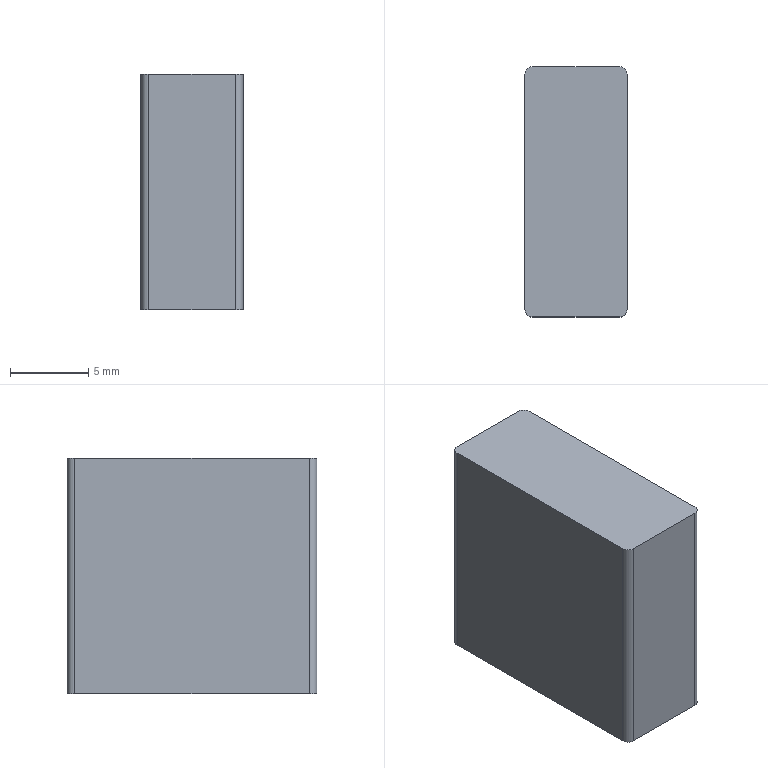Part | NX | features BREP 1 | 1 solid | 10 faces | box 6.52 x 15.946 x 15 mm | volume 1556 mm3 | plane 6 | cylinder 4 | commonest cylinder face diameters 1 x4
STEP:
#1=CARTESIAN_POINT('',(-2.76,7.973,-25.6));
#2=VERTEX_POINT('',#1);
#3=CARTESIAN_POINT('',(-3.26,7.473,-25.6));
#4=VERTEX_POINT('',#3);
#5=CARTESIAN_POINT('',(-2.76,7.473,-25.6));
#6=DIRECTION('',(0.,0.,1.));
#7=DIRECTION('',(1.,0.,0.));
#8=AXIS2_PLACEMENT_3D('',#5,#6,#7);
#9=CIRCLE('',#8,0.5);
#10=EDGE_CURVE('',#2,#4,#9,.T.);
#11=ORIENTED_EDGE('',*,*,#10,.F.);
#12=CARTESIAN_POINT('',(-2.76,7.973,-40.6));
#13=VERTEX_POINT('',#12);
#14=CARTESIAN_POINT('',(-2.76,7.973,-40.6));
#15=DIRECTION('',(0.,0.,1.));
#16=VECTOR('',#15,1000.);
#17=LINE('',#14,#16);
#18=EDGE_CURVE('',#13,#2,#17,.T.);
#19=ORIENTED_EDGE('',*,*,#18,.F.);
#20=CARTESIAN_POINT('',(-3.26,7.473,-40.6));
#21=VERTEX_POINT('',#20);
#22=CARTESIAN_POINT('',(-2.76,7.473,-40.6));
#23=DIRECTION('',(0.,0.,1.));
#24=DIRECTION('',(1.,0.,0.));
#25=AXIS2_PLACEMENT_3D('',#22,#23,#24);
#26=CIRCLE('',#25,0.5);
#27=EDGE_CURVE('',#13,#21,#26,.T.);
#28=ORIENTED_EDGE('',*,*,#27,.T.);
#29=CARTESIAN_POINT('',(-3.26,7.473,-40.6));
#30=DIRECTION('',(0.,0.,1.));
#31=VECTOR('',#30,1000.);
#32=LINE('',#29,#31);
#33=EDGE_CURVE('',#21,#4,#32,.T.);
#34=ORIENTED_EDGE('',*,*,#33,.T.);
#35=EDGE_LOOP('',(#11,#19,#28,#34));
#36=FACE_BOUND('',#35,.T.);
#37=CARTESIAN_POINT('',(-2.76,7.473,-40.6));
#38=DIRECTION('',(0.,0.,1.));
#39=DIRECTION('',(-1.,0.,0.));
#40=AXIS2_PLACEMENT_3D('',#37,#38,#39);
#41=CYLINDRICAL_SURFACE('',#40,0.5);
#42=ADVANCED_FACE('',(#36),#41,.T.);
#43=CARTESIAN_POINT('',(-3.26,-7.473,-25.6));
#44=VERTEX_POINT('',#43);
#45=CARTESIAN_POINT('',(-3.26,-7.473,-25.6));
#46=DIRECTION('',(0.,1.,0.));
#47=VECTOR('',#46,1000.);
#48=LINE('',#45,#47);
#49=EDGE_CURVE('',#44,#4,#48,.T.);
#50=ORIENTED_EDGE('',*,*,#49,.T.);
#51=ORIENTED_EDGE('',*,*,#33,.F.);
#52=CARTESIAN_POINT('',(-3.26,-7.473,-40.6));
#53=VERTEX_POINT('',#52);
#54=CARTESIAN_POINT('',(-3.26,-7.473,-40.6));
#55=DIRECTION('',(0.,1.,0.));
#56=VECTOR('',#55,1000.);
#57=LINE('',#54,#56);
#58=EDGE_CURVE('',#53,#21,#57,.T.);
#59=ORIENTED_EDGE('',*,*,#58,.F.);
#60=CARTESIAN_POINT('',(-3.26,-7.473,-40.6));
#61=DIRECTION('',(0.,0.,1.));
#62=VECTOR('',#61,1000.);
#63=LINE('',#60,#62);
#64=EDGE_CURVE('',#53,#44,#63,.T.);
#65=ORIENTED_EDGE('',*,*,#64,.T.);
#66=EDGE_LOOP('',(#50,#51,#59,#65));
#67=FACE_BOUND('',#66,.T.);
#68=CARTESIAN_POINT('',(-3.26,-7.473,-40.6));
#69=DIRECTION('',(1.,0.,0.));
#70=DIRECTION('',(0.,-1.,0.));
#71=AXIS2_PLACEMENT_3D('',#68,#69,#70);
#72=PLANE('',#71);
#73=ADVANCED_FACE('',(#67),#72,.F.);
#74=CARTESIAN_POINT('',(-2.76,-7.973,-25.6));
#75=VERTEX_POINT('',#74);
#76=CARTESIAN_POINT('',(-2.76,-7.473,-25.6));
#77=DIRECTION('',(0.,0.,1.));
#78=DIRECTION('',(1.,0.,0.));
#79=AXIS2_PLACEMENT_3D('',#76,#77,#78);
#80=CIRCLE('',#79,0.5);
#81=EDGE_CURVE('',#44,#75,#80,.T.);
#82=ORIENTED_EDGE('',*,*,#81,.F.);
#83=ORIENTED_EDGE('',*,*,#64,.F.);
#84=CARTESIAN_POINT('',(-2.76,-7.973,-40.6));
#85=VERTEX_POINT('',#84);
#86=CARTESIAN_POINT('',(-2.76,-7.473,-40.6));
#87=DIRECTION('',(0.,0.,1.));
#88=DIRECTION('',(1.,0.,0.));
#89=AXIS2_PLACEMENT_3D('',#86,#87,#88);
#90=CIRCLE('',#89,0.5);
#91=EDGE_CURVE('',#53,#85,#90,.T.);
#92=ORIENTED_EDGE('',*,*,#91,.T.);
#93=CARTESIAN_POINT('',(-2.76,-7.973,-40.6));
#94=DIRECTION('',(0.,0.,1.));
#95=VECTOR('',#94,1000.);
#96=LINE('',#93,#95);
#97=EDGE_CURVE('',#85,#75,#96,.T.);
#98=ORIENTED_EDGE('',*,*,#97,.T.);
#99=EDGE_LOOP('',(#82,#83,#92,#98));
#100=FACE_BOUND('',#99,.T.);
#101=CARTESIAN_POINT('',(-2.76,-7.473,-40.6));
#102=DIRECTION('',(0.,0.,1.));
#103=DIRECTION('',(-1.,0.,0.));
#104=AXIS2_PLACEMENT_3D('',#101,#102,#103);
#105=CYLINDRICAL_SURFACE('',#104,0.5);
#106=ADVANCED_FACE('',(#100),#105,.T.);
#107=CARTESIAN_POINT('',(2.76,-7.973,-25.6));
#108=VERTEX_POINT('',#107);
#109=CARTESIAN_POINT('',(2.76,-7.973,-25.6));
#110=DIRECTION('',(-1.,0.,0.));
#111=VECTOR('',#110,1000.);
#112=LINE('',#109,#111);
#113=EDGE_CURVE('',#108,#75,#112,.T.);
#114=ORIENTED_EDGE('',*,*,#113,.T.);
#115=ORIENTED_EDGE('',*,*,#97,.F.);
#116=CARTESIAN_POINT('',(2.76,-7.973,-40.6));
#117=VERTEX_POINT('',#116);
#118=CARTESIAN_POINT('',(2.76,-7.973,-40.6));
#119=DIRECTION('',(-1.,0.,0.));
#120=VECTOR('',#119,1000.);
#121=LINE('',#118,#120);
#122=EDGE_CURVE('',#117,#85,#121,.T.);
#123=ORIENTED_EDGE('',*,*,#122,.F.);
#124=CARTESIAN_POINT('',(2.76,-7.973,-40.6));
#125=DIRECTION('',(0.,0.,1.));
#126=VECTOR('',#125,1000.);
#127=LINE('',#124,#126);
#128=EDGE_CURVE('',#117,#108,#127,.T.);
#129=ORIENTED_EDGE('',*,*,#128,.T.);
#130=EDGE_LOOP('',(#114,#115,#123,#129));
#131=FACE_BOUND('',#130,.T.);
#132=CARTESIAN_POINT('',(2.76,-7.973,-40.6));
#133=DIRECTION('',(0.,1.,0.));
#134=DIRECTION('',(0.,0.,-1.));
#135=AXIS2_PLACEMENT_3D('',#132,#133,#134);
#136=PLANE('',#135);
#137=ADVANCED_FACE('',(#131),#136,.F.);
#138=CARTESIAN_POINT('',(3.26,-7.473,-25.6));
#139=VERTEX_POINT('',#138);
#140=CARTESIAN_POINT('',(2.76,-7.473,-25.6));
#141=DIRECTION('',(0.,0.,1.));
#142=DIRECTION('',(1.,0.,0.));
#143=AXIS2_PLACEMENT_3D('',#140,#141,#142);
#144=CIRCLE('',#143,0.5);
#145=EDGE_CURVE('',#108,#139,#144,.T.);
#146=ORIENTED_EDGE('',*,*,#145,.F.);
#147=ORIENTED_EDGE('',*,*,#128,.F.);
#148=CARTESIAN_POINT('',(3.26,-7.473,-40.6));
#149=VERTEX_POINT('',#148);
#150=CARTESIAN_POINT('',(2.76,-7.473,-40.6));
#151=DIRECTION('',(0.,0.,1.));
#152=DIRECTION('',(1.,0.,0.));
#153=AXIS2_PLACEMENT_3D('',#150,#151,#152);
#154=CIRCLE('',#153,0.5);
#155=EDGE_CURVE('',#117,#149,#154,.T.);
#156=ORIENTED_EDGE('',*,*,#155,.T.);
#157=CARTESIAN_POINT('',(3.26,-7.473,-40.6));
#158=DIRECTION('',(0.,0.,1.));
#159=VECTOR('',#158,1000.);
#160=LINE('',#157,#159);
#161=EDGE_CURVE('',#149,#139,#160,.T.);
#162=ORIENTED_EDGE('',*,*,#161,.T.);
#163=EDGE_LOOP('',(#146,#147,#156,#162));
#164=FACE_BOUND('',#163,.T.);
#165=CARTESIAN_POINT('',(2.76,-7.473,-40.6));
#166=DIRECTION('',(0.,0.,1.));
#167=DIRECTION('',(-1.,0.,0.));
#168=AXIS2_PLACEMENT_3D('',#165,#166,#167);
#169=CYLINDRICAL_SURFACE('',#168,0.5);
#170=ADVANCED_FACE('',(#164),#169,.T.);
#171=CARTESIAN_POINT('',(3.26,7.473,-25.6));
#172=VERTEX_POINT('',#171);
#173=CARTESIAN_POINT('',(3.26,7.473,-25.6));
#174=DIRECTION('',(0.,-1.,0.));
#175=VECTOR('',#174,1000.);
#176=LINE('',#173,#175);
#177=EDGE_CURVE('',#172,#139,#176,.T.);
#178=ORIENTED_EDGE('',*,*,#177,.T.);
#179=ORIENTED_EDGE('',*,*,#161,.F.);
#180=CARTESIAN_POINT('',(3.26,7.473,-40.6));
#181=VERTEX_POINT('',#180);
#182=CARTESIAN_POINT('',(3.26,7.473,-40.6));
#183=DIRECTION('',(0.,-1.,0.));
#184=VECTOR('',#183,1000.);
#185=LINE('',#182,#184);
#186=EDGE_CURVE('',#181,#149,#185,.T.);
#187=ORIENTED_EDGE('',*,*,#186,.F.);
#188=CARTESIAN_POINT('',(3.26,7.473,-40.6));
#189=DIRECTION('',(0.,0.,1.));
#190=VECTOR('',#189,1000.);
#191=LINE('',#188,#190);
#192=EDGE_CURVE('',#181,#172,#191,.T.);
#193=ORIENTED_EDGE('',*,*,#192,.T.);
#194=EDGE_LOOP('',(#178,#179,#187,#193));
#195=FACE_BOUND('',#194,.T.);
#196=CARTESIAN_POINT('',(3.26,7.473,-40.6));
#197=DIRECTION('',(-1.,0.,0.));
#198=DIRECTION('',(0.,0.,-1.));
#199=AXIS2_PLACEMENT_3D('',#196,#197,#198);
#200=PLANE('',#199);
#201=ADVANCED_FACE('',(#195),#200,.F.);
#202=CARTESIAN_POINT('',(2.76,7.973,-25.6));
#203=VERTEX_POINT('',#202);
#204=CARTESIAN_POINT('',(2.76,7.473,-25.6));
#205=DIRECTION('',(0.,0.,1.));
#206=DIRECTION('',(1.,0.,0.));
#207=AXIS2_PLACEMENT_3D('',#204,#205,#206);
#208=CIRCLE('',#207,0.5);
#209=EDGE_CURVE('',#172,#203,#208,.T.);
#210=ORIENTED_EDGE('',*,*,#209,.F.);
#211=ORIENTED_EDGE('',*,*,#192,.F.);
#212=CARTESIAN_POINT('',(2.76,7.973,-40.6));
#213=VERTEX_POINT('',#212);
#214=CARTESIAN_POINT('',(2.76,7.473,-40.6));
#215=DIRECTION('',(0.,0.,1.));
#216=DIRECTION('',(1.,0.,0.));
#217=AXIS2_PLACEMENT_3D('',#214,#215,#216);
#218=CIRCLE('',#217,0.5);
#219=EDGE_CURVE('',#181,#213,#218,.T.);
#220=ORIENTED_EDGE('',*,*,#219,.T.);
#221=CARTESIAN_POINT('',(2.76,7.973,-40.6));
#222=DIRECTION('',(0.,0.,1.));
#223=VECTOR('',#222,1000.);
#224=LINE('',#221,#223);
#225=EDGE_CURVE('',#213,#203,#224,.T.);
#226=ORIENTED_EDGE('',*,*,#225,.T.);
#227=EDGE_LOOP('',(#210,#211,#220,#226));
#228=FACE_BOUND('',#227,.T.);
#229=CARTESIAN_POINT('',(2.76,7.473,-40.6));
#230=DIRECTION('',(0.,0.,1.));
#231=DIRECTION('',(-1.,0.,0.));
#232=AXIS2_PLACEMENT_3D('',#229,#230,#231);
#233=CYLINDRICAL_SURFACE('',#232,0.5);
#234=ADVANCED_FACE('',(#228),#233,.T.);
#235=CARTESIAN_POINT('',(-2.76,7.973,-25.6));
#236=DIRECTION('',(1.,0.,0.));
#237=VECTOR('',#236,1000.);
#238=LINE('',#235,#237);
#239=EDGE_CURVE('',#2,#203,#238,.T.);
#240=ORIENTED_EDGE('',*,*,#239,.T.);
#241=ORIENTED_EDGE('',*,*,#225,.F.);
#242=CARTESIAN_POINT('',(-2.76,7.973,-40.6));
#243=DIRECTION('',(1.,0.,0.));
#244=VECTOR('',#243,1000.);
#245=LINE('',#242,#244);
#246=EDGE_CURVE('',#13,#213,#245,.T.);
#247=ORIENTED_EDGE('',*,*,#246,.F.);
#248=ORIENTED_EDGE('',*,*,#18,.T.);
#249=EDGE_LOOP('',(#240,#241,#247,#248));
#250=FACE_BOUND('',#249,.T.);
#251=CARTESIAN_POINT('',(-2.76,7.973,-40.6));
#252=DIRECTION('',(0.,-1.,0.));
#253=DIRECTION('',(0.,0.,1.));
#254=AXIS2_PLACEMENT_3D('',#251,#252,#253);
#255=PLANE('',#254);
#256=ADVANCED_FACE('',(#250),#255,.F.);
#257=ORIENTED_EDGE('',*,*,#27,.F.);
#258=ORIENTED_EDGE('',*,*,#246,.T.);
#259=ORIENTED_EDGE('',*,*,#219,.F.);
#260=ORIENTED_EDGE('',*,*,#186,.T.);
#261=ORIENTED_EDGE('',*,*,#155,.F.);
#262=ORIENTED_EDGE('',*,*,#122,.T.);
#263=ORIENTED_EDGE('',*,*,#91,.F.);
#264=ORIENTED_EDGE('',*,*,#58,.T.);
#265=EDGE_LOOP('',(#257,#258,#259,#260,#261,#262,#263,#264));
#266=FACE_BOUND('',#265,.T.);
#267=CARTESIAN_POINT('',(-2.76,7.473,-40.6));
#268=DIRECTION('',(0.,0.,1.));
#269=DIRECTION('',(-1.,0.,0.));
#270=AXIS2_PLACEMENT_3D('',#267,#268,#269);
#271=PLANE('',#270);
#272=ADVANCED_FACE('',(#266),#271,.F.);
#273=ORIENTED_EDGE('',*,*,#10,.T.);
#274=ORIENTED_EDGE('',*,*,#49,.F.);
#275=ORIENTED_EDGE('',*,*,#81,.T.);
#276=ORIENTED_EDGE('',*,*,#113,.F.);
#277=ORIENTED_EDGE('',*,*,#145,.T.);
#278=ORIENTED_EDGE('',*,*,#177,.F.);
#279=ORIENTED_EDGE('',*,*,#209,.T.);
#280=ORIENTED_EDGE('',*,*,#239,.F.);
#281=EDGE_LOOP('',(#273,#274,#275,#276,#277,#278,#279,#280));
#282=FACE_BOUND('',#281,.T.);
#283=CARTESIAN_POINT('',(-2.76,7.473,-25.6));
#284=DIRECTION('',(0.,0.,1.));
#285=DIRECTION('',(-1.,0.,0.));
#286=AXIS2_PLACEMENT_3D('',#283,#284,#285);
#287=PLANE('',#286);
#288=ADVANCED_FACE('',(#282),#287,.T.);
#289=CLOSED_SHELL('',(#42,#73,#106,#137,#170,#201,#234,#256,#272,#288));
#290=MANIFOLD_SOLID_BREP('',#289);
#291=(LENGTH_UNIT()NAMED_UNIT(*)SI_UNIT(.MILLI.,.METRE.));
#292=UNCERTAINTY_MEASURE_WITH_UNIT(LENGTH_MEASURE(0.00001),#291,'','');
#293=(NAMED_UNIT(*)PLANE_ANGLE_UNIT()SI_UNIT($,.RADIAN.));
#294=(NAMED_UNIT(*)SI_UNIT($,.STERADIAN.)SOLID_ANGLE_UNIT());
#295=(GEOMETRIC_REPRESENTATION_CONTEXT(3)GLOBAL_UNCERTAINTY_ASSIGNED_CONTEXT((#292))GLOBAL_UNIT_ASSIGNED_CONTEXT((#291,#293,#294))REPRESENTATION_CONTEXT('',''));
#296=ADVANCED_BREP_SHAPE_REPRESENTATION('',(#290),#295);